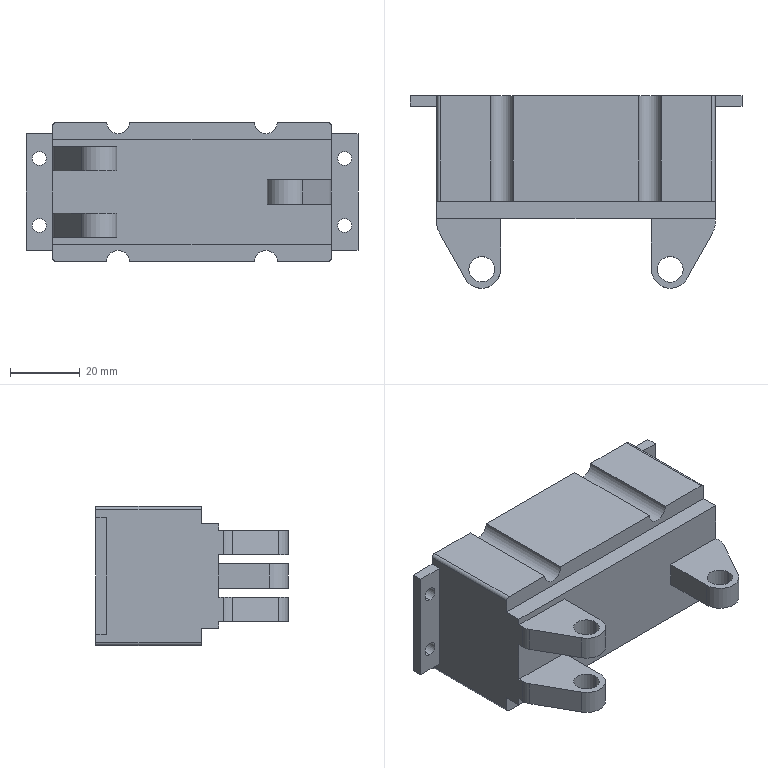Part | SolidWorks | features ICE 4, Cut 1, Extrusion 1, Fillet 1, MirrorPattern 1 | 1 solid | 64 faces | box 95.251 x 55.228 x 40 mm | volume 112954 mm3 | plane 34 | cylinder 30 | commonest cylinder face diameters 4 x8 6.492 x6 7.349 x6 2 x4 10 x3 10.89 x3